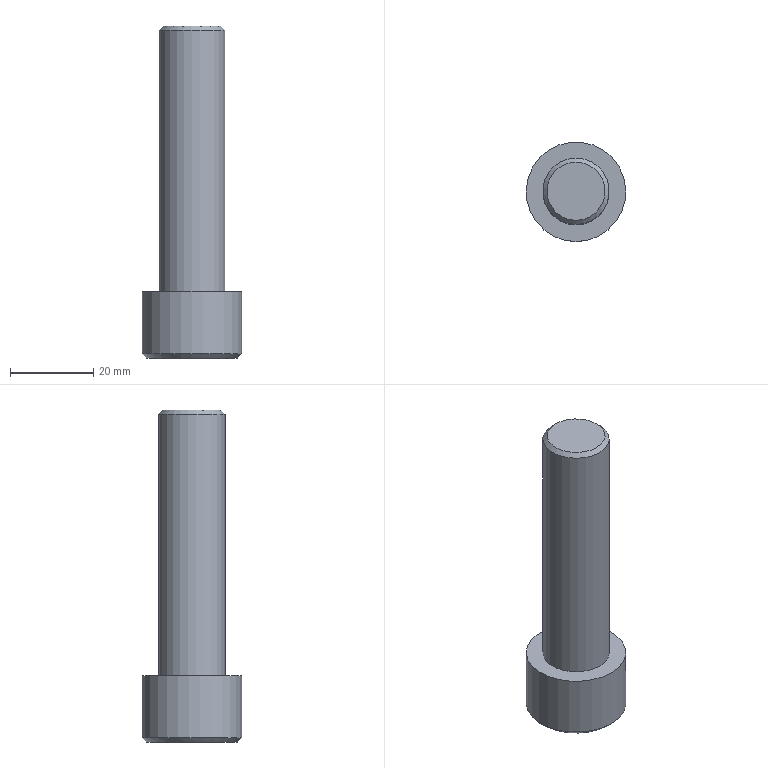Part | STEP file | solid 221 | 1 solid | 14 faces | box 24 x 24 x 80 mm | volume 18857 mm3 | plane 10 | cylinder 2 | cone 2 | commonest cylinder face diameters 16 x1 24 x1